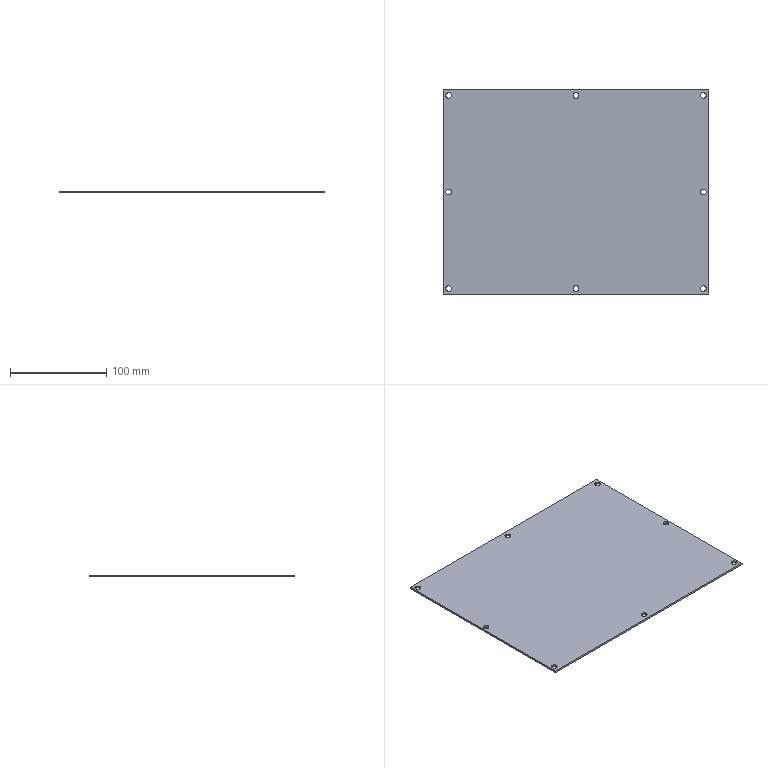Part | STEP file | Rear guard plate SGN-7-04 | 1 solid | 22 faces | box 274 x 213 x 2 mm | volume 116272 mm3 | cylinder 16 | plane 6 | commonest cylinder face diameters 6 x16